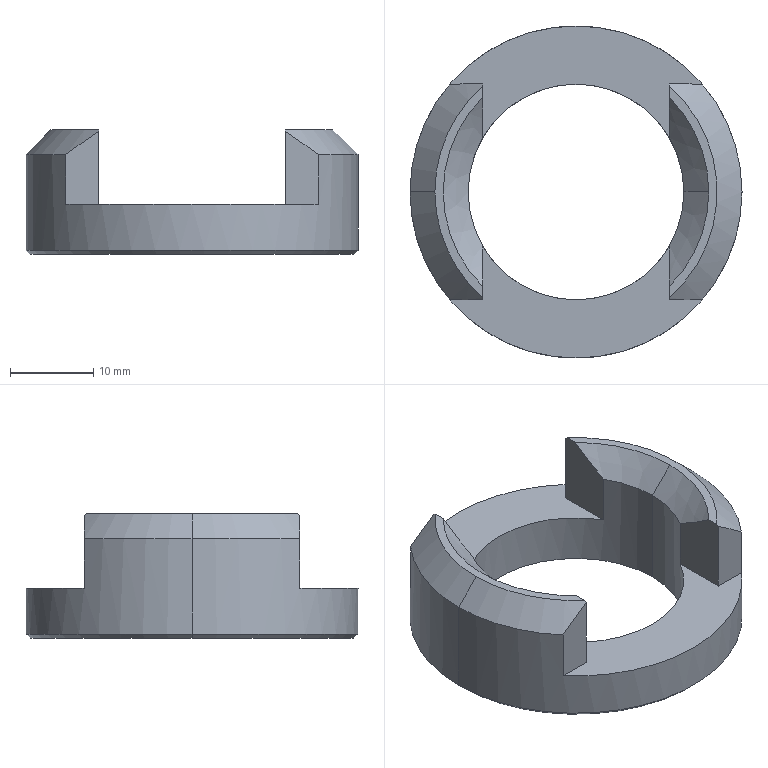Part | NX | 1 solid | 41 faces | box 40 x 40 x 15 mm | volume 6938 mm3 | cone 16 | plane 13 | cylinder 12 | commonest cylinder face diameters 2.5 x8 26 x2 40 x2